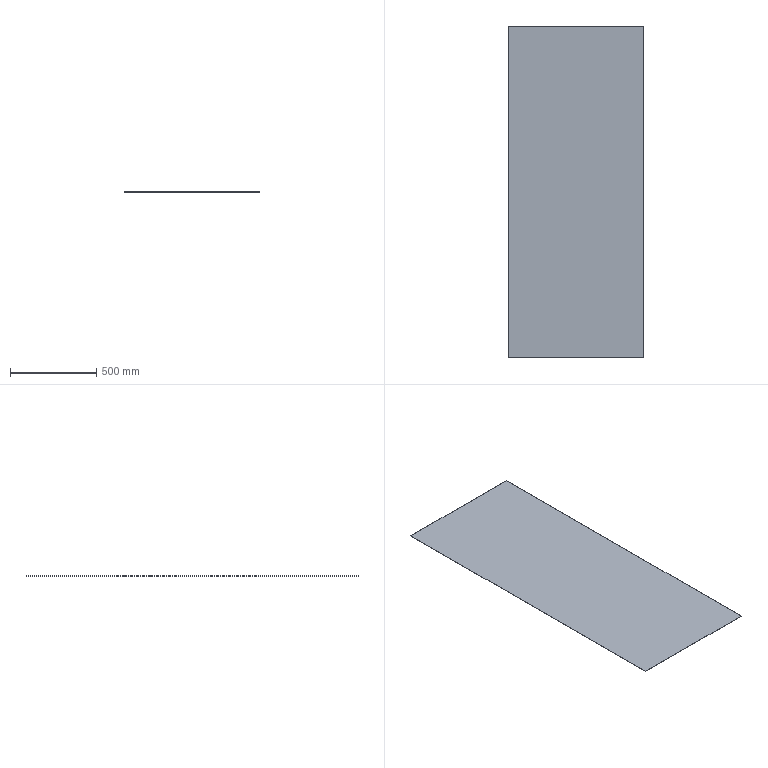Part | STEP file | 750038414 | 1 solid | 6 faces | box 785 x 1925 x 1.5 mm | volume 2266688 mm3 | plane 6
STEP:
#1=CARTESIAN_POINT('',(-392.5,-962.5,1.5));
#2=VERTEX_POINT('',#1);
#3=CARTESIAN_POINT('',(392.5,-962.5,1.5));
#4=VERTEX_POINT('',#3);
#5=CARTESIAN_POINT('',(0.,-962.5,1.5));
#6=DIRECTION('',(1.,0.,0.));
#7=VECTOR('',#6,1000.);
#8=LINE('',#5,#7);
#9=EDGE_CURVE('',#2,#4,#8,.T.);
#10=ORIENTED_EDGE('',*,*,#9,.T.);
#11=CARTESIAN_POINT('',(392.5,962.5,1.5));
#12=VERTEX_POINT('',#11);
#13=CARTESIAN_POINT('',(392.5,0.,1.5));
#14=DIRECTION('',(0.,1.,0.));
#15=VECTOR('',#14,1000.);
#16=LINE('',#13,#15);
#17=EDGE_CURVE('',#4,#12,#16,.T.);
#18=ORIENTED_EDGE('',*,*,#17,.T.);
#19=CARTESIAN_POINT('',(-392.5,962.5,1.5));
#20=VERTEX_POINT('',#19);
#21=CARTESIAN_POINT('',(0.,962.5,1.5));
#22=DIRECTION('',(-1.,0.,0.));
#23=VECTOR('',#22,1000.);
#24=LINE('',#21,#23);
#25=EDGE_CURVE('',#12,#20,#24,.T.);
#26=ORIENTED_EDGE('',*,*,#25,.T.);
#27=CARTESIAN_POINT('',(-392.5,0.,1.5));
#28=DIRECTION('',(0.,-1.,0.));
#29=VECTOR('',#28,1000.);
#30=LINE('',#27,#29);
#31=EDGE_CURVE('',#20,#2,#30,.T.);
#32=ORIENTED_EDGE('',*,*,#31,.T.);
#33=EDGE_LOOP('',(#10,#18,#26,#32));
#34=FACE_OUTER_BOUND('',#33,.T.);
#35=CARTESIAN_POINT('',(0.,0.,1.5));
#36=DIRECTION('',(0.,0.,1.));
#37=DIRECTION('',(1.,0.,0.));
#38=AXIS2_PLACEMENT_3D('',#35,#36,#37);
#39=PLANE('',#38);
#40=ADVANCED_FACE('',(#34),#39,.T.);
#41=CARTESIAN_POINT('',(392.5,962.5,0.));
#42=VERTEX_POINT('',#41);
#43=CARTESIAN_POINT('',(392.5,962.5,1.5));
#44=DIRECTION('',(0.,0.,-1.));
#45=VECTOR('',#44,1000.);
#46=LINE('',#43,#45);
#47=EDGE_CURVE('',#12,#42,#46,.T.);
#48=ORIENTED_EDGE('',*,*,#47,.F.);
#49=ORIENTED_EDGE('',*,*,#17,.F.);
#50=CARTESIAN_POINT('',(392.5,-962.5,0.));
#51=VERTEX_POINT('',#50);
#52=CARTESIAN_POINT('',(392.5,-962.5,1.5));
#53=DIRECTION('',(0.,0.,1.));
#54=VECTOR('',#53,1000.);
#55=LINE('',#52,#54);
#56=EDGE_CURVE('',#51,#4,#55,.T.);
#57=ORIENTED_EDGE('',*,*,#56,.F.);
#58=CARTESIAN_POINT('',(392.5,-962.5,0.));
#59=DIRECTION('',(0.,-1.,0.));
#60=VECTOR('',#59,1000.);
#61=LINE('',#58,#60);
#62=EDGE_CURVE('',#42,#51,#61,.T.);
#63=ORIENTED_EDGE('',*,*,#62,.F.);
#64=EDGE_LOOP('',(#48,#49,#57,#63));
#65=FACE_OUTER_BOUND('',#64,.T.);
#66=CARTESIAN_POINT('',(392.5,-962.5,1.5));
#67=DIRECTION('',(-1.,0.,0.));
#68=DIRECTION('',(0.,0.,1.));
#69=AXIS2_PLACEMENT_3D('',#66,#67,#68);
#70=PLANE('',#69);
#71=ADVANCED_FACE('',(#65),#70,.F.);
#72=ORIENTED_EDGE('',*,*,#56,.T.);
#73=ORIENTED_EDGE('',*,*,#9,.F.);
#74=CARTESIAN_POINT('',(-392.5,-962.5,0.));
#75=VERTEX_POINT('',#74);
#76=CARTESIAN_POINT('',(-392.5,-962.5,1.5));
#77=DIRECTION('',(0.,0.,1.));
#78=VECTOR('',#77,1000.);
#79=LINE('',#76,#78);
#80=EDGE_CURVE('',#75,#2,#79,.T.);
#81=ORIENTED_EDGE('',*,*,#80,.F.);
#82=CARTESIAN_POINT('',(-392.5,-962.5,0.));
#83=DIRECTION('',(-1.,0.,0.));
#84=VECTOR('',#83,1000.);
#85=LINE('',#82,#84);
#86=EDGE_CURVE('',#51,#75,#85,.T.);
#87=ORIENTED_EDGE('',*,*,#86,.F.);
#88=EDGE_LOOP('',(#72,#73,#81,#87));
#89=FACE_OUTER_BOUND('',#88,.T.);
#90=CARTESIAN_POINT('',(-392.5,-962.5,1.5));
#91=DIRECTION('',(0.,1.,0.));
#92=DIRECTION('',(0.,0.,1.));
#93=AXIS2_PLACEMENT_3D('',#90,#91,#92);
#94=PLANE('',#93);
#95=ADVANCED_FACE('',(#89),#94,.F.);
#96=ORIENTED_EDGE('',*,*,#80,.T.);
#97=ORIENTED_EDGE('',*,*,#31,.F.);
#98=CARTESIAN_POINT('',(-392.5,962.5,0.));
#99=VERTEX_POINT('',#98);
#100=CARTESIAN_POINT('',(-392.5,962.5,1.5));
#101=DIRECTION('',(0.,0.,1.));
#102=VECTOR('',#101,1000.);
#103=LINE('',#100,#102);
#104=EDGE_CURVE('',#99,#20,#103,.T.);
#105=ORIENTED_EDGE('',*,*,#104,.F.);
#106=CARTESIAN_POINT('',(-392.5,962.5,0.));
#107=DIRECTION('',(0.,1.,0.));
#108=VECTOR('',#107,1000.);
#109=LINE('',#106,#108);
#110=EDGE_CURVE('',#75,#99,#109,.T.);
#111=ORIENTED_EDGE('',*,*,#110,.F.);
#112=EDGE_LOOP('',(#96,#97,#105,#111));
#113=FACE_OUTER_BOUND('',#112,.T.);
#114=CARTESIAN_POINT('',(-392.5,962.5,1.5));
#115=DIRECTION('',(1.,0.,0.));
#116=DIRECTION('',(0.,0.,-1.));
#117=AXIS2_PLACEMENT_3D('',#114,#115,#116);
#118=PLANE('',#117);
#119=ADVANCED_FACE('',(#113),#118,.F.);
#120=ORIENTED_EDGE('',*,*,#104,.T.);
#121=ORIENTED_EDGE('',*,*,#25,.F.);
#122=ORIENTED_EDGE('',*,*,#47,.T.);
#123=CARTESIAN_POINT('',(392.5,962.5,0.));
#124=DIRECTION('',(1.,0.,0.));
#125=VECTOR('',#124,1000.);
#126=LINE('',#123,#125);
#127=EDGE_CURVE('',#99,#42,#126,.T.);
#128=ORIENTED_EDGE('',*,*,#127,.F.);
#129=EDGE_LOOP('',(#120,#121,#122,#128));
#130=FACE_OUTER_BOUND('',#129,.T.);
#131=CARTESIAN_POINT('',(392.5,962.5,1.5));
#132=DIRECTION('',(0.,-1.,0.));
#133=DIRECTION('',(0.,0.,-1.));
#134=AXIS2_PLACEMENT_3D('',#131,#132,#133);
#135=PLANE('',#134);
#136=ADVANCED_FACE('',(#130),#135,.F.);
#137=ORIENTED_EDGE('',*,*,#62,.T.);
#138=ORIENTED_EDGE('',*,*,#86,.T.);
#139=ORIENTED_EDGE('',*,*,#110,.T.);
#140=ORIENTED_EDGE('',*,*,#127,.T.);
#141=EDGE_LOOP('',(#137,#138,#139,#140));
#142=FACE_OUTER_BOUND('',#141,.T.);
#143=CARTESIAN_POINT('',(0.,0.,0.));
#144=DIRECTION('',(0.,0.,1.));
#145=DIRECTION('',(1.,0.,0.));
#146=AXIS2_PLACEMENT_3D('',#143,#144,#145);
#147=PLANE('',#146);
#148=ADVANCED_FACE('',(#142),#147,.F.);
#149=CLOSED_SHELL('',(#40,#71,#95,#119,#136,#148));
#150=MANIFOLD_SOLID_BREP('',#149);
#151=CARTESIAN_POINT('',(0.,0.,0.));
#152=DIRECTION('',(0.,0.,1.));
#153=DIRECTION('',(1.,0.,0.));
#154=AXIS2_PLACEMENT_3D('',#151,#152,#153);
#155=(LENGTH_UNIT()NAMED_UNIT(*)SI_UNIT(.MILLI.,.METRE.));
#156=UNCERTAINTY_MEASURE_WITH_UNIT(LENGTH_MEASURE(0.00001),#155,'','');
#157=(NAMED_UNIT(*)PLANE_ANGLE_UNIT()SI_UNIT($,.RADIAN.));
#158=(NAMED_UNIT(*)SI_UNIT($,.STERADIAN.)SOLID_ANGLE_UNIT());
#159=(GEOMETRIC_REPRESENTATION_CONTEXT(3)GLOBAL_UNCERTAINTY_ASSIGNED_CONTEXT((#156))GLOBAL_UNIT_ASSIGNED_CONTEXT((#155,#157,#158))REPRESENTATION_CONTEXT('',''));
#160=ADVANCED_BREP_SHAPE_REPRESENTATION('',(#150,#154),#159);